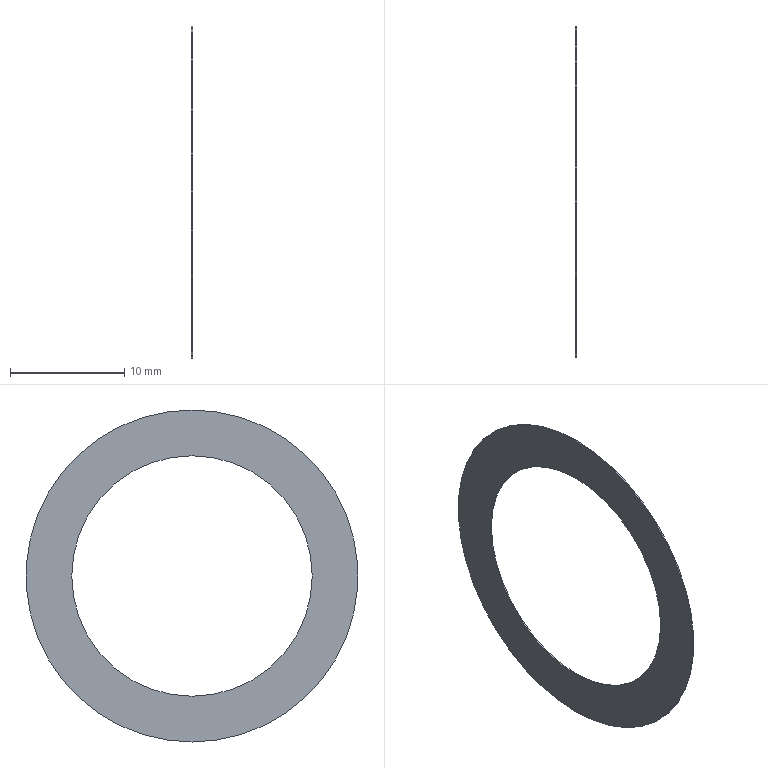Part | NX | features solid 2 | 1 solid | 6 faces | box 0.1 x 29 x 29 mm | volume 31.416 mm3 | cylinder 4 | plane 2 | commonest cylinder face diameters 21 x2 29 x2
STEP:
#1=CARTESIAN_POINT('',(166.2,-71.5,-968.5));
#2=VERTEX_POINT('',#1);
#3=CARTESIAN_POINT('',(166.2,-71.5,-939.5));
#4=VERTEX_POINT('',#3);
#5=CARTESIAN_POINT('',(166.2,-71.5,-954.));
#6=DIRECTION('',(-1.,0.,0.));
#7=DIRECTION('',(0.,0.,-1.));
#8=AXIS2_PLACEMENT_3D('',#5,#6,#7);
#9=CIRCLE('',#8,14.5);
#10=EDGE_CURVE('',#2,#4,#9,.T.);
#11=ORIENTED_EDGE('',*,*,#10,.F.);
#12=CARTESIAN_POINT('',(166.2,-71.5,-954.));
#13=DIRECTION('',(-1.,0.,0.));
#14=DIRECTION('',(0.,0.,1.));
#15=AXIS2_PLACEMENT_3D('',#12,#13,#14);
#16=CIRCLE('',#15,14.5);
#17=EDGE_CURVE('',#4,#2,#16,.T.);
#18=ORIENTED_EDGE('',*,*,#17,.F.);
#19=EDGE_LOOP('',(#11,#18));
#20=FACE_BOUND('',#19,.T.);
#21=CARTESIAN_POINT('',(166.2,-71.5,-943.5));
#22=VERTEX_POINT('',#21);
#23=CARTESIAN_POINT('',(166.2,-71.5,-964.5));
#24=VERTEX_POINT('',#23);
#25=CARTESIAN_POINT('',(166.2,-71.5,-954.));
#26=DIRECTION('',(1.,0.,0.));
#27=DIRECTION('',(0.,0.,1.));
#28=AXIS2_PLACEMENT_3D('',#25,#26,#27);
#29=CIRCLE('',#28,10.5);
#30=EDGE_CURVE('',#22,#24,#29,.T.);
#31=ORIENTED_EDGE('',*,*,#30,.F.);
#32=CARTESIAN_POINT('',(166.2,-71.5,-954.));
#33=DIRECTION('',(1.,0.,0.));
#34=DIRECTION('',(0.,0.,-1.));
#35=AXIS2_PLACEMENT_3D('',#32,#33,#34);
#36=CIRCLE('',#35,10.5);
#37=EDGE_CURVE('',#24,#22,#36,.T.);
#38=ORIENTED_EDGE('',*,*,#37,.F.);
#39=EDGE_LOOP('',(#31,#38));
#40=FACE_BOUND('',#39,.T.);
#41=CARTESIAN_POINT('',(166.2,-71.5,-954.));
#42=DIRECTION('',(-1.,0.,0.));
#43=DIRECTION('',(0.,0.,-1.));
#44=AXIS2_PLACEMENT_3D('',#41,#42,#43);
#45=PLANE('',#44);
#46=ADVANCED_FACE('',(#20,#40),#45,.F.);
#47=CARTESIAN_POINT('',(166.1,-71.5,-968.5));
#48=VERTEX_POINT('',#47);
#49=CARTESIAN_POINT('',(166.1,-71.5,-968.5));
#50=DIRECTION('',(1.,0.,0.));
#51=VECTOR('',#50,1000.);
#52=LINE('',#49,#51);
#53=EDGE_CURVE('',#48,#2,#52,.T.);
#54=ORIENTED_EDGE('',*,*,#53,.F.);
#55=CARTESIAN_POINT('',(166.1,-71.5,-939.5));
#56=VERTEX_POINT('',#55);
#57=CARTESIAN_POINT('',(166.1,-71.5,-954.));
#58=DIRECTION('',(1.,0.,0.));
#59=DIRECTION('',(0.,0.,-1.));
#60=AXIS2_PLACEMENT_3D('',#57,#58,#59);
#61=CIRCLE('',#60,14.5);
#62=EDGE_CURVE('',#48,#56,#61,.T.);
#63=ORIENTED_EDGE('',*,*,#62,.T.);
#64=CARTESIAN_POINT('',(166.1,-71.5,-939.5));
#65=DIRECTION('',(1.,0.,0.));
#66=VECTOR('',#65,1000.);
#67=LINE('',#64,#66);
#68=EDGE_CURVE('',#4,#56,#67,.F.);
#69=ORIENTED_EDGE('',*,*,#68,.F.);
#70=ORIENTED_EDGE('',*,*,#17,.T.);
#71=EDGE_LOOP('',(#54,#63,#69,#70));
#72=FACE_BOUND('',#71,.T.);
#73=CARTESIAN_POINT('',(166.2,-71.5,-954.));
#74=DIRECTION('',(-1.,0.,0.));
#75=DIRECTION('',(0.,0.,-1.));
#76=AXIS2_PLACEMENT_3D('',#73,#74,#75);
#77=CYLINDRICAL_SURFACE('',#76,14.5);
#78=ADVANCED_FACE('',(#72),#77,.T.);
#79=ORIENTED_EDGE('',*,*,#10,.T.);
#80=ORIENTED_EDGE('',*,*,#68,.T.);
#81=CARTESIAN_POINT('',(166.1,-71.5,-954.));
#82=DIRECTION('',(1.,0.,0.));
#83=DIRECTION('',(0.,0.,1.));
#84=AXIS2_PLACEMENT_3D('',#81,#82,#83);
#85=CIRCLE('',#84,14.5);
#86=EDGE_CURVE('',#56,#48,#85,.T.);
#87=ORIENTED_EDGE('',*,*,#86,.T.);
#88=ORIENTED_EDGE('',*,*,#53,.T.);
#89=EDGE_LOOP('',(#79,#80,#87,#88));
#90=FACE_BOUND('',#89,.T.);
#91=CARTESIAN_POINT('',(166.2,-71.5,-954.));
#92=DIRECTION('',(-1.,0.,0.));
#93=DIRECTION('',(0.,0.,-1.));
#94=AXIS2_PLACEMENT_3D('',#91,#92,#93);
#95=CYLINDRICAL_SURFACE('',#94,14.5);
#96=ADVANCED_FACE('',(#90),#95,.T.);
#97=ORIENTED_EDGE('',*,*,#86,.F.);
#98=ORIENTED_EDGE('',*,*,#62,.F.);
#99=EDGE_LOOP('',(#97,#98));
#100=FACE_BOUND('',#99,.T.);
#101=CARTESIAN_POINT('',(166.1,-71.5,-964.5));
#102=VERTEX_POINT('',#101);
#103=CARTESIAN_POINT('',(166.1,-71.5,-943.5));
#104=VERTEX_POINT('',#103);
#105=CARTESIAN_POINT('',(166.1,-71.5,-954.));
#106=DIRECTION('',(-1.,0.,0.));
#107=DIRECTION('',(0.,0.,-1.));
#108=AXIS2_PLACEMENT_3D('',#105,#106,#107);
#109=CIRCLE('',#108,10.5);
#110=EDGE_CURVE('',#102,#104,#109,.T.);
#111=ORIENTED_EDGE('',*,*,#110,.F.);
#112=CARTESIAN_POINT('',(166.1,-71.5,-954.));
#113=DIRECTION('',(-1.,0.,0.));
#114=DIRECTION('',(0.,0.,1.));
#115=AXIS2_PLACEMENT_3D('',#112,#113,#114);
#116=CIRCLE('',#115,10.5);
#117=EDGE_CURVE('',#104,#102,#116,.T.);
#118=ORIENTED_EDGE('',*,*,#117,.F.);
#119=EDGE_LOOP('',(#111,#118));
#120=FACE_BOUND('',#119,.T.);
#121=CARTESIAN_POINT('',(166.1,-71.5,-954.));
#122=DIRECTION('',(-1.,0.,0.));
#123=DIRECTION('',(0.,0.,-1.));
#124=AXIS2_PLACEMENT_3D('',#121,#122,#123);
#125=PLANE('',#124);
#126=ADVANCED_FACE('',(#100,#120),#125,.T.);
#127=ORIENTED_EDGE('',*,*,#37,.T.);
#128=CARTESIAN_POINT('',(166.1,-71.5,-943.5));
#129=DIRECTION('',(1.,0.,0.));
#130=VECTOR('',#129,1000.);
#131=LINE('',#128,#130);
#132=EDGE_CURVE('',#104,#22,#131,.T.);
#133=ORIENTED_EDGE('',*,*,#132,.F.);
#134=ORIENTED_EDGE('',*,*,#117,.T.);
#135=CARTESIAN_POINT('',(166.1,-71.5,-964.5));
#136=DIRECTION('',(1.,0.,0.));
#137=VECTOR('',#136,1000.);
#138=LINE('',#135,#137);
#139=EDGE_CURVE('',#24,#102,#138,.F.);
#140=ORIENTED_EDGE('',*,*,#139,.F.);
#141=EDGE_LOOP('',(#127,#133,#134,#140));
#142=FACE_BOUND('',#141,.T.);
#143=CARTESIAN_POINT('',(166.2,-71.5,-954.));
#144=DIRECTION('',(-1.,0.,0.));
#145=DIRECTION('',(0.,0.,-1.));
#146=AXIS2_PLACEMENT_3D('',#143,#144,#145);
#147=CYLINDRICAL_SURFACE('',#146,10.5);
#148=ADVANCED_FACE('',(#142),#147,.F.);
#149=ORIENTED_EDGE('',*,*,#139,.T.);
#150=ORIENTED_EDGE('',*,*,#110,.T.);
#151=ORIENTED_EDGE('',*,*,#132,.T.);
#152=ORIENTED_EDGE('',*,*,#30,.T.);
#153=EDGE_LOOP('',(#149,#150,#151,#152));
#154=FACE_BOUND('',#153,.T.);
#155=CARTESIAN_POINT('',(166.2,-71.5,-954.));
#156=DIRECTION('',(-1.,0.,0.));
#157=DIRECTION('',(0.,0.,-1.));
#158=AXIS2_PLACEMENT_3D('',#155,#156,#157);
#159=CYLINDRICAL_SURFACE('',#158,10.5);
#160=ADVANCED_FACE('',(#154),#159,.F.);
#161=CLOSED_SHELL('',(#46,#78,#96,#126,#148,#160));
#162=MANIFOLD_SOLID_BREP('',#161);
#163=(LENGTH_UNIT()NAMED_UNIT(*)SI_UNIT(.MILLI.,.METRE.));
#164=UNCERTAINTY_MEASURE_WITH_UNIT(LENGTH_MEASURE(0.00001),#163,'','');
#165=(NAMED_UNIT(*)PLANE_ANGLE_UNIT()SI_UNIT($,.RADIAN.));
#166=(NAMED_UNIT(*)SI_UNIT($,.STERADIAN.)SOLID_ANGLE_UNIT());
#167=(GEOMETRIC_REPRESENTATION_CONTEXT(3)GLOBAL_UNCERTAINTY_ASSIGNED_CONTEXT((#164))GLOBAL_UNIT_ASSIGNED_CONTEXT((#163,#165,#166))REPRESENTATION_CONTEXT('',''));
#168=ADVANCED_BREP_SHAPE_REPRESENTATION('',(#162),#167);